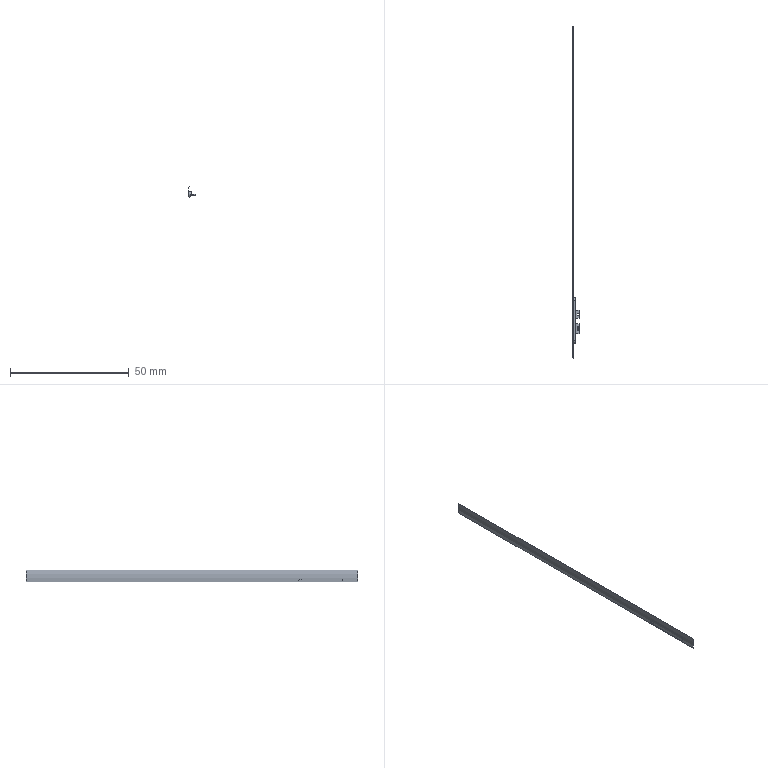Part | Creo | 1 solid | 43 faces | box 2.96 x 139.6 x 4.9 mm | volume 378.881 mm3 | plane 23 | cylinder 20 | commonest cylinder face diameters 0.4 x4 0.547 x4 1.1 x4 1 x2 1.3 x2 2.1 x2